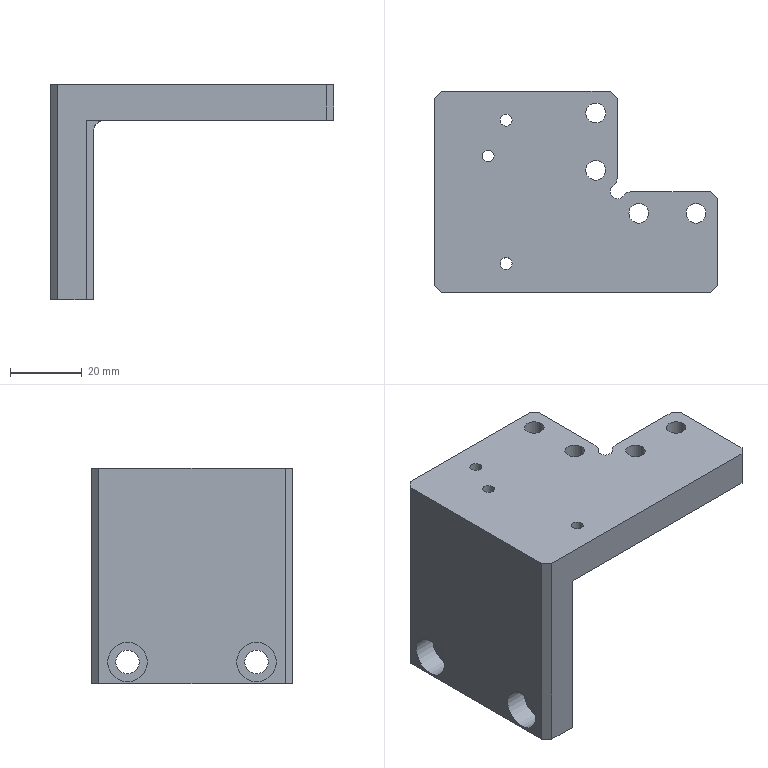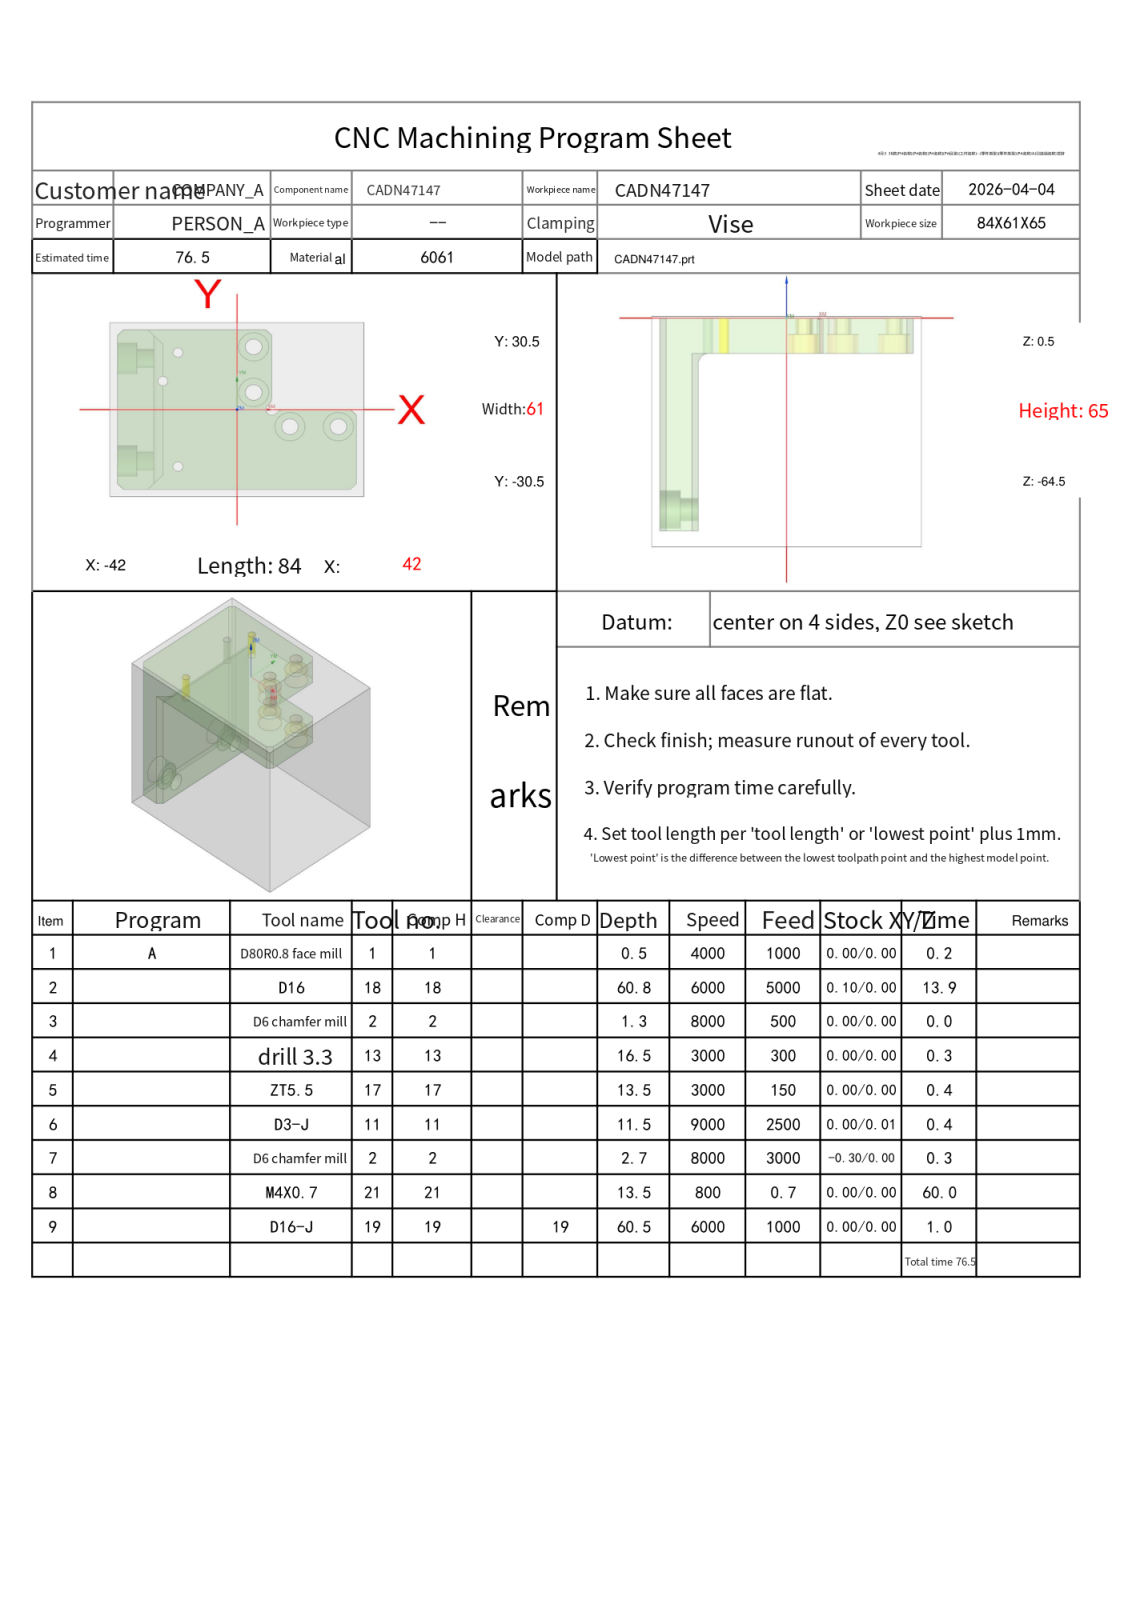NC program | NX | posted by the shop | part box 79 x 56 x 60 mm
Lines 7245 to 9053 of 9053, first 1638 of 1809 lines:
N3 T02 M06
(D6 chamfer mill  D=6. R=0. H=02 ce=0.00 di=0.00)
G00 G90 G54 X-19.5 Y-20. M03 S8000
G43 H02 Z20.
M08
G98 G81 X-19.5 Y-20. Z-.8 R1. F500.
X-24.5 Y10.
X-19.5 Y20.
X5.5 Y22.
Y6.
X17.5 Y-6.
X33.5
G80
G00 Z20.
G91 G28 Z0.0
M05
M09
G91 G28 Z0.0
M01
N4 T13 M06
(drill 3.3 D=3.3 DR_a=118 H=13)
G00 G90 G54 X-19.5 Y-20. M03 S3000
G43 H13 Z20.
M08
G98 G83 X-19.5 Y-20. Z-15.991 R1. F300. Q2.
Y20.
G80
G00 Z20.
G00 G90 X-24.5 Y10. M03 S3000
Z20.
G98 G83 X-24.5 Y10. Z-16. R1. F120. Q2.
G80
G00 Z20.
G91 G28 Z0.0
M05
M09
G91 G28 Z0.0
M01
N5 T17 M06
(ZT5.5 D=5.5 DR_a=118 H=17)
G00 G90 G54 X33.5 Y-6. M03 S3000
G43 H17 Z20.
M08
G98 G83 X33.5 Y-6. Z-13. R1. F150. Q3.
X17.5
X5.5 Y6.
Y22.
G80
G00 Z20.
G91 G28 Z0.0
M05
M09
G91 G28 Z0.0
M01
N6 T11 M06
(D3-J  D=3. R=0. H=11 ce=0.00 di=0.01)
G00 G90 G54 X13.577 Y9.224 M03 S9000
G43 H11 Z20.
M08
Z.153
G01 X13.571 Y9.223 Z.084 F2000.
X13.553 Y9.221 Z.023
X13.527 Y9.216 Z-.032
X13.491 Y9.21 Z-.081
X13.45 Y9.202 Z-.124
X13.403 Y9.191 Z-.161
X13.353 Y9.177 Z-.193
X13.3 Y9.161 Z-.22
X13.247 Y9.142 Z-.243
X13.195 Y9.119 Z-.261
X13.145 Y9.093 Z-.275
X13.099 Y9.064 Z-.285
X13.059 Y9.03 Z-.292
X13.025 Y8.993 Z-.296
X13. Y8.952 Z-.297
Y4. F2500.
G02 X11.2 Y.4 I-4.5 J0.0
G03 X11. Y0.0 I.3 J-.4
X11.5 Y-.5 I.5 J0.0
X11.9 Y-.3 I0.0 J.5
G02 X15.5 Y1.5 I3.6 J-2.7
G01 X20.452
X20.493 Y1.525 Z-.296
X20.53 Y1.559 Z-.292
X20.564 Y1.599 Z-.285
X20.593 Y1.645 Z-.275
X20.619 Y1.695 Z-.261
X20.642 Y1.747 Z-.243
X20.661 Y1.8 Z-.22
X20.677 Y1.853 Z-.193
X20.691 Y1.903 Z-.161
X20.702 Y1.95 Z-.124
X20.71 Y1.991 Z-.081
X20.716 Y2.027 Z-.032
X20.721 Y2.053 Z.023
X20.723 Y2.071 Z.084
X20.724 Y2.077 Z.153
G00 Z3.
X13.577 Y9.224
Z-.145
G01 X13.571 Y9.223 Z-.213 F2000.
X13.553 Y9.221 Z-.275
X13.527 Y9.216 Z-.33
X13.491 Y9.21 Z-.378
X13.45 Y9.202 Z-.421
X13.403 Y9.191 Z-.459
X13.353 Y9.177 Z-.49
X13.3 Y9.161 Z-.518
X13.247 Y9.142 Z-.54
X13.195 Y9.119 Z-.558
X13.145 Y9.093 Z-.572
X13.099 Y9.064 Z-.582
X13.059 Y9.03 Z-.589
X13.025 Y8.993 Z-.593
X13. Y8.952 Z-.595
Y4. F2500.
G02 X11.2 Y.4 I-4.5 J0.0
G03 X11. Y0.0 I.3 J-.4
X11.5 Y-.5 I.5 J0.0
X11.9 Y-.3 I0.0 J.5
G02 X15.5 Y1.5 I3.6 J-2.7
G01 X20.452
X20.493 Y1.525 Z-.593
X20.53 Y1.559 Z-.589
X20.564 Y1.599 Z-.582
X20.593 Y1.645 Z-.572
X20.619 Y1.695 Z-.558
X20.642 Y1.747 Z-.54
X20.661 Y1.8 Z-.518
X20.677 Y1.853 Z-.49
X20.691 Y1.903 Z-.459
X20.702 Y1.95 Z-.421
X20.71 Y1.991 Z-.378
X20.716 Y2.027 Z-.33
X20.721 Y2.053 Z-.275
X20.723 Y2.071 Z-.213
X20.724 Y2.077 Z-.145
G00 Z2.703
X13.577 Y9.224
Z-.442
G01 X13.571 Y9.223 Z-.51 F2000.
X13.553 Y9.221 Z-.572
X13.527 Y9.216 Z-.627
X13.491 Y9.21 Z-.676
X13.45 Y9.202 Z-.719
X13.403 Y9.191 Z-.756
X13.353 Y9.177 Z-.788
X13.3 Y9.161 Z-.815
X13.247 Y9.142 Z-.837
X13.195 Y9.119 Z-.855
X13.145 Y9.093 Z-.869
X13.099 Y9.064 Z-.88
X13.059 Y9.03 Z-.887
X13.025 Y8.993 Z-.891
X13. Y8.952 Z-.892
Y4. F2500.
G02 X11.2 Y.4 I-4.5 J0.0
G03 X11. Y0.0 I.3 J-.4
X11.5 Y-.5 I.5 J0.0
X11.9 Y-.3 I0.0 J.5
G02 X15.5 Y1.5 I3.6 J-2.7
G01 X20.452
X20.493 Y1.525 Z-.891
X20.53 Y1.559 Z-.887
X20.564 Y1.599 Z-.88
X20.593 Y1.645 Z-.869
X20.619 Y1.695 Z-.855
X20.642 Y1.747 Z-.837
X20.661 Y1.8 Z-.815
X20.677 Y1.853 Z-.788
X20.691 Y1.903 Z-.756
X20.702 Y1.95 Z-.719
X20.71 Y1.991 Z-.676
X20.716 Y2.027 Z-.627
X20.721 Y2.053 Z-.572
X20.723 Y2.071 Z-.51
X20.724 Y2.077 Z-.442
G00 Z2.405
X13.577 Y9.224
Z-.739
G01 X13.571 Y9.223 Z-.808 F2000.
X13.553 Y9.221 Z-.869
X13.527 Y9.216 Z-.924
X13.491 Y9.21 Z-.973
X13.45 Y9.202 Z-1.016
X13.403 Y9.191 Z-1.053
X13.353 Y9.177 Z-1.085
X13.3 Y9.161 Z-1.112
X13.247 Y9.142 Z-1.134
X13.195 Y9.119 Z-1.153
X13.145 Y9.093 Z-1.167
X13.099 Y9.064 Z-1.177
X13.059 Y9.03 Z-1.184
X13.025 Y8.993 Z-1.188
X13. Y8.952 Z-1.189
Y4. F2500.
G02 X11.2 Y.4 I-4.5 J0.0
G03 X11. Y0.0 I.3 J-.4
X11.5 Y-.5 I.5 J0.0
X11.9 Y-.3 I0.0 J.5
G02 X15.5 Y1.5 I3.6 J-2.7
G01 X20.452
X20.493 Y1.525 Z-1.188
X20.53 Y1.559 Z-1.184
X20.564 Y1.599 Z-1.177
X20.593 Y1.645 Z-1.167
X20.619 Y1.695 Z-1.153
X20.642 Y1.747 Z-1.134
X20.661 Y1.8 Z-1.112
X20.677 Y1.853 Z-1.085
X20.691 Y1.903 Z-1.053
X20.702 Y1.95 Z-1.016
X20.71 Y1.991 Z-.973
X20.716 Y2.027 Z-.924
X20.721 Y2.053 Z-.869
X20.723 Y2.071 Z-.808
X20.724 Y2.077 Z-.739
G00 Z2.108
X13.577 Y9.224
Z-1.036
G01 X13.571 Y9.223 Z-1.105 F2000.
X13.553 Y9.221 Z-1.167
X13.527 Y9.216 Z-1.222
X13.491 Y9.21 Z-1.27
X13.45 Y9.202 Z-1.313
X13.403 Y9.191 Z-1.35
X13.353 Y9.177 Z-1.382
X13.3 Y9.161 Z-1.409
X13.247 Y9.142 Z-1.432
X13.195 Y9.119 Z-1.45
X13.145 Y9.093 Z-1.464
X13.099 Y9.064 Z-1.474
X13.059 Y9.03 Z-1.481
X13.025 Y8.993 Z-1.485
X13. Y8.952 Z-1.486
Y4. F2500.
G02 X11.2 Y.4 I-4.5 J0.0
G03 X11. Y0.0 I.3 J-.4
X11.5 Y-.5 I.5 J0.0
X11.9 Y-.3 I0.0 J.5
G02 X15.5 Y1.5 I3.6 J-2.7
G01 X20.452
X20.493 Y1.525 Z-1.485
X20.53 Y1.559 Z-1.481
X20.564 Y1.599 Z-1.474
X20.593 Y1.645 Z-1.464
X20.619 Y1.695 Z-1.45
X20.642 Y1.747 Z-1.432
X20.661 Y1.8 Z-1.409
X20.677 Y1.853 Z-1.382
X20.691 Y1.903 Z-1.35
X20.702 Y1.95 Z-1.313
X20.71 Y1.991 Z-1.27
X20.716 Y2.027 Z-1.222
X20.721 Y2.053 Z-1.167
X20.723 Y2.071 Z-1.105
X20.724 Y2.077 Z-1.036
G00 Z1.811
X13.577 Y9.224
Z-1.334
G01 X13.571 Y9.223 Z-1.402 F2000.
X13.553 Y9.221 Z-1.464
X13.527 Y9.216 Z-1.519
X13.491 Y9.21 Z-1.568
X13.45 Y9.202 Z-1.61
X13.403 Y9.191 Z-1.648
X13.353 Y9.177 Z-1.68
X13.3 Y9.161 Z-1.707
X13.247 Y9.142 Z-1.729
X13.195 Y9.119 Z-1.747
X13.145 Y9.093 Z-1.761
X13.099 Y9.064 Z-1.772
X13.059 Y9.03 Z-1.779
X13.025 Y8.993 Z-1.783
X13. Y8.952 Z-1.784
Y4. F2500.
G02 X11.2 Y.4 I-4.5 J0.0
G03 X11. Y0.0 I.3 J-.4
X11.5 Y-.5 I.5 J0.0
X11.9 Y-.3 I0.0 J.5
G02 X15.5 Y1.5 I3.6 J-2.7
G01 X20.452
X20.493 Y1.525 Z-1.783
X20.53 Y1.559 Z-1.779
X20.564 Y1.599 Z-1.772
X20.593 Y1.645 Z-1.761
X20.619 Y1.695 Z-1.747
X20.642 Y1.747 Z-1.729
X20.661 Y1.8 Z-1.707
X20.677 Y1.853 Z-1.68
X20.691 Y1.903 Z-1.648
X20.702 Y1.95 Z-1.61
X20.71 Y1.991 Z-1.568
X20.716 Y2.027 Z-1.519
X20.721 Y2.053 Z-1.464
X20.723 Y2.071 Z-1.402
X20.724 Y2.077 Z-1.334
G00 Z1.514
X13.577 Y9.224
Z-1.631
G01 X13.571 Y9.223 Z-1.7 F2000.
X13.553 Y9.221 Z-1.761
X13.527 Y9.216 Z-1.816
X13.491 Y9.21 Z-1.865
X13.45 Y9.202 Z-1.908
X13.403 Y9.191 Z-1.945
X13.353 Y9.177 Z-1.977
X13.3 Y9.161 Z-2.004
X13.247 Y9.142 Z-2.026
X13.195 Y9.119 Z-2.044
X13.145 Y9.093 Z-2.058
X13.099 Y9.064 Z-2.069
X13.059 Y9.03 Z-2.076
X13.025 Y8.993 Z-2.08
X13. Y8.952 Z-2.081
Y4. F2500.
G02 X11.2 Y.4 I-4.5 J0.0
G03 X11. Y0.0 I.3 J-.4
X11.5 Y-.5 I.5 J0.0
X11.9 Y-.3 I0.0 J.5
G02 X15.5 Y1.5 I3.6 J-2.7
G01 X20.452
X20.493 Y1.525 Z-2.08
X20.53 Y1.559 Z-2.076
X20.564 Y1.599 Z-2.069
X20.593 Y1.645 Z-2.058
X20.619 Y1.695 Z-2.044
X20.642 Y1.747 Z-2.026
X20.661 Y1.8 Z-2.004
X20.677 Y1.853 Z-1.977
X20.691 Y1.903 Z-1.945
X20.702 Y1.95 Z-1.908
X20.71 Y1.991 Z-1.865
X20.716 Y2.027 Z-1.816
X20.721 Y2.053 Z-1.761
X20.723 Y2.071 Z-1.7
X20.724 Y2.077 Z-1.631
G00 Z1.216
X13.577 Y9.224
Z-1.928
G01 X13.571 Y9.223 Z-1.997 F2000.
X13.553 Y9.221 Z-2.058
X13.527 Y9.216 Z-2.113
X13.491 Y9.21 Z-2.162
X13.45 Y9.202 Z-2.205
X13.403 Y9.191 Z-2.242
X13.353 Y9.177 Z-2.274
X13.3 Y9.161 Z-2.301
X13.247 Y9.142 Z-2.324
X13.195 Y9.119 Z-2.342
X13.145 Y9.093 Z-2.356
X13.099 Y9.064 Z-2.366
X13.059 Y9.03 Z-2.373
X13.025 Y8.993 Z-2.377
X13. Y8.952 Z-2.378
Y4. F2500.
G02 X11.2 Y.4 I-4.5 J0.0
G03 X11. Y0.0 I.3 J-.4
X11.5 Y-.5 I.5 J0.0
X11.9 Y-.3 I0.0 J.5
G02 X15.5 Y1.5 I3.6 J-2.7
G01 X20.452
X20.493 Y1.525 Z-2.377
X20.53 Y1.559 Z-2.373
X20.564 Y1.599 Z-2.366
X20.593 Y1.645 Z-2.356
X20.619 Y1.695 Z-2.342
X20.642 Y1.747 Z-2.324
X20.661 Y1.8 Z-2.301
X20.677 Y1.853 Z-2.274
X20.691 Y1.903 Z-2.242
X20.702 Y1.95 Z-2.205
X20.71 Y1.991 Z-2.162
X20.716 Y2.027 Z-2.113
X20.721 Y2.053 Z-2.058
X20.723 Y2.071 Z-1.997
X20.724 Y2.077 Z-1.928
G00 Z.919
X13.577 Y9.224
Z-2.226
G01 X13.571 Y9.223 Z-2.294 F2000.
X13.553 Y9.221 Z-2.356
X13.527 Y9.216 Z-2.411
X13.491 Y9.21 Z-2.459
X13.45 Y9.202 Z-2.502
X13.403 Y9.191 Z-2.54
X13.353 Y9.177 Z-2.572
X13.3 Y9.161 Z-2.599
X13.247 Y9.142 Z-2.621
X13.195 Y9.119 Z-2.639
X13.145 Y9.093 Z-2.653
X13.099 Y9.064 Z-2.663
X13.059 Y9.03 Z-2.67
X13.025 Y8.993 Z-2.674
X13. Y8.952 Z-2.676
Y4. F2500.
G02 X11.2 Y.4 I-4.5 J0.0
G03 X11. Y0.0 I.3 J-.4
X11.5 Y-.5 I.5 J0.0
X11.9 Y-.3 I0.0 J.5
G02 X15.5 Y1.5 I3.6 J-2.7
G01 X20.452
X20.493 Y1.525 Z-2.674
X20.53 Y1.559 Z-2.67
X20.564 Y1.599 Z-2.663
X20.593 Y1.645 Z-2.653
X20.619 Y1.695 Z-2.639
X20.642 Y1.747 Z-2.621
X20.661 Y1.8 Z-2.599
X20.677 Y1.853 Z-2.572
X20.691 Y1.903 Z-2.54
X20.702 Y1.95 Z-2.502
X20.71 Y1.991 Z-2.459
X20.716 Y2.027 Z-2.411
X20.721 Y2.053 Z-2.356
X20.723 Y2.071 Z-2.294
X20.724 Y2.077 Z-2.226
G00 Z.622
X13.577 Y9.224
Z-2.523
G01 X13.571 Y9.223 Z-2.591 F2000.
X13.553 Y9.221 Z-2.653
X13.527 Y9.216 Z-2.708
X13.491 Y9.21 Z-2.757
X13.45 Y9.202 Z-2.8
X13.403 Y9.191 Z-2.837
X13.353 Y9.177 Z-2.869
X13.3 Y9.161 Z-2.896
X13.247 Y9.142 Z-2.918
X13.195 Y9.119 Z-2.936
X13.145 Y9.093 Z-2.95
X13.099 Y9.064 Z-2.961
X13.059 Y9.03 Z-2.968
X13.025 Y8.993 Z-2.972
X13. Y8.952 Z-2.973
Y4. F2500.
G02 X11.2 Y.4 I-4.5 J0.0
G03 X11. Y0.0 I.3 J-.4
X11.5 Y-.5 I.5 J0.0
X11.9 Y-.3 I0.0 J.5
G02 X15.5 Y1.5 I3.6 J-2.7
G01 X20.452
X20.493 Y1.525 Z-2.972
X20.53 Y1.559 Z-2.968
X20.564 Y1.599 Z-2.961
X20.593 Y1.645 Z-2.95
X20.619 Y1.695 Z-2.936
X20.642 Y1.747 Z-2.918
X20.661 Y1.8 Z-2.896
X20.677 Y1.853 Z-2.869
X20.691 Y1.903 Z-2.837
X20.702 Y1.95 Z-2.8
X20.71 Y1.991 Z-2.757
X20.716 Y2.027 Z-2.708
X20.721 Y2.053 Z-2.653
X20.723 Y2.071 Z-2.591
X20.724 Y2.077 Z-2.523
G00 Z.324
X13.577 Y9.224
Z-2.82
G01 X13.571 Y9.223 Z-2.889 F2000.
X13.553 Y9.221 Z-2.95
X13.527 Y9.216 Z-3.005
X13.491 Y9.21 Z-3.054
X13.45 Y9.202 Z-3.097
X13.403 Y9.191 Z-3.134
X13.353 Y9.177 Z-3.166
X13.3 Y9.161 Z-3.193
X13.247 Y9.142 Z-3.216
X13.195 Y9.119 Z-3.234
X13.145 Y9.093 Z-3.248
X13.099 Y9.064 Z-3.258
X13.059 Y9.03 Z-3.265
X13.025 Y8.993 Z-3.269
X13. Y8.952 Z-3.27
Y4. F2500.
G02 X11.2 Y.4 I-4.5 J0.0
G03 X11. Y0.0 I.3 J-.4
X11.5 Y-.5 I.5 J0.0
X11.9 Y-.3 I0.0 J.5
G02 X15.5 Y1.5 I3.6 J-2.7
G01 X20.452
X20.493 Y1.525 Z-3.269
X20.53 Y1.559 Z-3.265
X20.564 Y1.599 Z-3.258
X20.593 Y1.645 Z-3.248
X20.619 Y1.695 Z-3.234
X20.642 Y1.747 Z-3.216
X20.661 Y1.8 Z-3.193
X20.677 Y1.853 Z-3.166
X20.691 Y1.903 Z-3.134
X20.702 Y1.95 Z-3.097
X20.71 Y1.991 Z-3.054
X20.716 Y2.027 Z-3.005
X20.721 Y2.053 Z-2.95
X20.723 Y2.071 Z-2.889
X20.724 Y2.077 Z-2.82
G00 Z.027
X13.577 Y9.224
Z-3.118
G01 X13.571 Y9.223 Z-3.186 F2000.
X13.553 Y9.221 Z-3.248
X13.527 Y9.216 Z-3.303
X13.491 Y9.21 Z-3.351
X13.45 Y9.202 Z-3.394
X13.403 Y9.191 Z-3.431
X13.353 Y9.177 Z-3.463
X13.3 Y9.161 Z-3.49
X13.247 Y9.142 Z-3.513
X13.195 Y9.119 Z-3.531
X13.145 Y9.093 Z-3.545
X13.099 Y9.064 Z-3.555
X13.059 Y9.03 Z-3.562
X13.025 Y8.993 Z-3.566
X13. Y8.952 Z-3.568
Y4. F2500.
G02 X11.2 Y.4 I-4.5 J0.0
G03 X11. Y0.0 I.3 J-.4
X11.5 Y-.5 I.5 J0.0
X11.9 Y-.3 I0.0 J.5
G02 X15.5 Y1.5 I3.6 J-2.7
G01 X20.452
X20.493 Y1.525 Z-3.566
X20.53 Y1.559 Z-3.562
X20.564 Y1.599 Z-3.555
X20.593 Y1.645 Z-3.545
X20.619 Y1.695 Z-3.531
X20.642 Y1.747 Z-3.513
X20.661 Y1.8 Z-3.49
X20.677 Y1.853 Z-3.463
X20.691 Y1.903 Z-3.431
X20.702 Y1.95 Z-3.394
X20.71 Y1.991 Z-3.351
X20.716 Y2.027 Z-3.303
X20.721 Y2.053 Z-3.248
X20.723 Y2.071 Z-3.186
X20.724 Y2.077 Z-3.118
G00 Z-.27
X13.577 Y9.224
Z-3.415
G01 X13.571 Y9.223 Z-3.483 F2000.
X13.553 Y9.221 Z-3.545
X13.527 Y9.216 Z-3.6
X13.491 Y9.21 Z-3.649
X13.45 Y9.202 Z-3.692
X13.403 Y9.191 Z-3.729
X13.353 Y9.177 Z-3.761
X13.3 Y9.161 Z-3.788
X13.247 Y9.142 Z-3.81
X13.195 Y9.119 Z-3.828
X13.145 Y9.093 Z-3.842
X13.099 Y9.064 Z-3.853
X13.059 Y9.03 Z-3.86
X13.025 Y8.993 Z-3.864
X13. Y8.952 Z-3.865
Y4. F2500.
G02 X11.2 Y.4 I-4.5 J0.0
G03 X11. Y0.0 I.3 J-.4
X11.5 Y-.5 I.5 J0.0
X11.9 Y-.3 I0.0 J.5
G02 X15.5 Y1.5 I3.6 J-2.7
G01 X20.452
X20.493 Y1.525 Z-3.864
X20.53 Y1.559 Z-3.86
X20.564 Y1.599 Z-3.853
X20.593 Y1.645 Z-3.842
X20.619 Y1.695 Z-3.828
X20.642 Y1.747 Z-3.81
X20.661 Y1.8 Z-3.788
X20.677 Y1.853 Z-3.761
X20.691 Y1.903 Z-3.729
X20.702 Y1.95 Z-3.692
X20.71 Y1.991 Z-3.649
X20.716 Y2.027 Z-3.6
X20.721 Y2.053 Z-3.545
X20.723 Y2.071 Z-3.483
X20.724 Y2.077 Z-3.415
G00 Z-.568
X13.577 Y9.224
Z-3.712
G01 X13.571 Y9.223 Z-3.781 F2000.
X13.553 Y9.221 Z-3.842
X13.527 Y9.216 Z-3.897
X13.491 Y9.21 Z-3.946
X13.45 Y9.202 Z-3.989
X13.403 Y9.191 Z-4.026
X13.353 Y9.177 Z-4.058
X13.3 Y9.161 Z-4.085
X13.247 Y9.142 Z-4.107
X13.195 Y9.119 Z-4.125
X13.145 Y9.093 Z-4.14
X13.099 Y9.064 Z-4.15
X13.059 Y9.03 Z-4.157
X13.025 Y8.993 Z-4.161
X13. Y8.952 Z-4.162
Y4. F2500.
G02 X11.2 Y.4 I-4.5 J0.0
G03 X11. Y0.0 I.3 J-.4
X11.5 Y-.5 I.5 J0.0
X11.9 Y-.3 I0.0 J.5
G02 X15.5 Y1.5 I3.6 J-2.7
G01 X20.452
X20.493 Y1.525 Z-4.161
X20.53 Y1.559 Z-4.157
X20.564 Y1.599 Z-4.15
X20.593 Y1.645 Z-4.14
X20.619 Y1.695 Z-4.125
X20.642 Y1.747 Z-4.107
X20.661 Y1.8 Z-4.085
X20.677 Y1.853 Z-4.058
X20.691 Y1.903 Z-4.026
X20.702 Y1.95 Z-3.989
X20.71 Y1.991 Z-3.946
X20.716 Y2.027 Z-3.897
X20.721 Y2.053 Z-3.842
X20.723 Y2.071 Z-3.781
X20.724 Y2.077 Z-3.712
G00 Z-.865
X13.577 Y9.224
Z-4.009
G01 X13.571 Y9.223 Z-4.078 F2000.
X13.553 Y9.221 Z-4.139
X13.527 Y9.216 Z-4.195
X13.491 Y9.21 Z-4.243
X13.45 Y9.202 Z-4.286
X13.403 Y9.191 Z-4.323
X13.353 Y9.177 Z-4.355
X13.3 Y9.161 Z-4.382
X13.247 Y9.142 Z-4.405
X13.195 Y9.119 Z-4.423
X13.145 Y9.093 Z-4.437
X13.099 Y9.064 Z-4.447
X13.059 Y9.03 Z-4.454
X13.025 Y8.993 Z-4.458
X13. Y8.952 Z-4.459
Y4. F2500.
G02 X11.2 Y.4 I-4.5 J0.0
G03 X11. Y0.0 I.3 J-.4
X11.5 Y-.5 I.5 J0.0
X11.9 Y-.3 I0.0 J.5
G02 X15.5 Y1.5 I3.6 J-2.7
G01 X20.452
X20.493 Y1.525 Z-4.458
X20.53 Y1.559 Z-4.454
X20.564 Y1.599 Z-4.447
X20.593 Y1.645 Z-4.437
X20.619 Y1.695 Z-4.423
X20.642 Y1.747 Z-4.405
X20.661 Y1.8 Z-4.382
X20.677 Y1.853 Z-4.355
X20.691 Y1.903 Z-4.323
X20.702 Y1.95 Z-4.286
X20.71 Y1.991 Z-4.243
X20.716 Y2.027 Z-4.195
X20.721 Y2.053 Z-4.139
X20.723 Y2.071 Z-4.078
X20.724 Y2.077 Z-4.009
G00 Z-1.162
X13.577 Y9.224
Z-4.307
G01 X13.571 Y9.223 Z-4.375 F2000.
X13.553 Y9.221 Z-4.437
X13.527 Y9.216 Z-4.492
X13.491 Y9.21 Z-4.541
X13.45 Y9.202 Z-4.583
X13.403 Y9.191 Z-4.621
X13.353 Y9.177 Z-4.653
X13.3 Y9.161 Z-4.68
X13.247 Y9.142 Z-4.702
X13.195 Y9.119 Z-4.72
X13.145 Y9.093 Z-4.734
X13.099 Y9.064 Z-4.745
X13.059 Y9.03 Z-4.752
X13.025 Y8.993 Z-4.756
X13. Y8.952 Z-4.757
Y4. F2500.
G02 X11.2 Y.4 I-4.5 J0.0
G03 X11. Y0.0 I.3 J-.4
X11.5 Y-.5 I.5 J0.0
X11.9 Y-.3 I0.0 J.5
G02 X15.5 Y1.5 I3.6 J-2.7
G01 X20.452
X20.493 Y1.525 Z-4.756
X20.53 Y1.559 Z-4.752
X20.564 Y1.599 Z-4.745
X20.593 Y1.645 Z-4.734
X20.619 Y1.695 Z-4.72
X20.642 Y1.747 Z-4.702
X20.661 Y1.8 Z-4.68
X20.677 Y1.853 Z-4.653
X20.691 Y1.903 Z-4.621
X20.702 Y1.95 Z-4.583
X20.71 Y1.991 Z-4.541
X20.716 Y2.027 Z-4.492
X20.721 Y2.053 Z-4.437
X20.723 Y2.071 Z-4.375
X20.724 Y2.077 Z-4.307
G00 Z-1.459
X13.577 Y9.224
Z-4.604
G01 X13.571 Y9.223 Z-4.673 F2000.
X13.553 Y9.221 Z-4.734
X13.527 Y9.216 Z-4.789
X13.491 Y9.21 Z-4.838
X13.45 Y9.202 Z-4.881
X13.403 Y9.191 Z-4.918
X13.353 Y9.177 Z-4.95
X13.3 Y9.161 Z-4.977
X13.247 Y9.142 Z-4.999
X13.195 Y9.119 Z-5.017
X13.145 Y9.093 Z-5.031
X13.099 Y9.064 Z-5.042
X13.059 Y9.03 Z-5.049
X13.025 Y8.993 Z-5.053
X13. Y8.952 Z-5.054
Y4. F2500.
G02 X11.2 Y.4 I-4.5 J0.0
G03 X11. Y0.0 I.3 J-.4
X11.5 Y-.5 I.5 J0.0
X11.9 Y-.3 I0.0 J.5
G02 X15.5 Y1.5 I3.6 J-2.7
G01 X20.452
X20.493 Y1.525 Z-5.053
X20.53 Y1.559 Z-5.049
X20.564 Y1.599 Z-5.042
X20.593 Y1.645 Z-5.031
X20.619 Y1.695 Z-5.017
X20.642 Y1.747 Z-4.999
X20.661 Y1.8 Z-4.977
X20.677 Y1.853 Z-4.95
X20.691 Y1.903 Z-4.918
X20.702 Y1.95 Z-4.881
X20.71 Y1.991 Z-4.838
X20.716 Y2.027 Z-4.789
X20.721 Y2.053 Z-4.734
X20.723 Y2.071 Z-4.673
X20.724 Y2.077 Z-4.604
G00 Z-1.757
X13.577 Y9.224
Z-4.901
G01 X13.571 Y9.223 Z-4.97 F2000.
X13.553 Y9.221 Z-5.031
X13.527 Y9.216 Z-5.086
X13.491 Y9.21 Z-5.135
X13.45 Y9.202 Z-5.178
X13.403 Y9.191 Z-5.215
X13.353 Y9.177 Z-5.247
X13.3 Y9.161 Z-5.274
X13.247 Y9.142 Z-5.297
X13.195 Y9.119 Z-5.315
X13.145 Y9.093 Z-5.329
X13.099 Y9.064 Z-5.339
X13.059 Y9.03 Z-5.346
X13.025 Y8.993 Z-5.35
X13. Y8.952 Z-5.351
Y4. F2500.
G02 X11.2 Y.4 I-4.5 J0.0
G03 X11. Y0.0 I.3 J-.4
X11.5 Y-.5 I.5 J0.0
X11.9 Y-.3 I0.0 J.5
G02 X15.5 Y1.5 I3.6 J-2.7
G01 X20.452
X20.493 Y1.525 Z-5.35
X20.53 Y1.559 Z-5.346
X20.564 Y1.599 Z-5.339
X20.593 Y1.645 Z-5.329
X20.619 Y1.695 Z-5.315
X20.642 Y1.747 Z-5.297
X20.661 Y1.8 Z-5.274
X20.677 Y1.853 Z-5.247
X20.691 Y1.903 Z-5.215
X20.702 Y1.95 Z-5.178
X20.71 Y1.991 Z-5.135
X20.716 Y2.027 Z-5.086
X20.721 Y2.053 Z-5.031
X20.723 Y2.071 Z-4.97
X20.724 Y2.077 Z-4.901
G00 Z-2.054
X13.577 Y9.224
Z-5.199
G01 X13.571 Y9.223 Z-5.267 F2000.
X13.553 Y9.221 Z-5.329
X13.527 Y9.216 Z-5.384
X13.491 Y9.21 Z-5.432
X13.45 Y9.202 Z-5.475
X13.403 Y9.191 Z-5.513
X13.353 Y9.177 Z-5.545
X13.3 Y9.161 Z-5.572
X13.247 Y9.142 Z-5.594
X13.195 Y9.119 Z-5.612
X13.145 Y9.093 Z-5.626
X13.099 Y9.064 Z-5.636
X13.059 Y9.03 Z-5.643
X13.025 Y8.993 Z-5.647
X13. Y8.952 Z-5.649
Y4. F2500.
G02 X11.2 Y.4 I-4.5 J0.0
G03 X11. Y0.0 I.3 J-.4
X11.5 Y-.5 I.5 J0.0
X11.9 Y-.3 I0.0 J.5
G02 X15.5 Y1.5 I3.6 J-2.7
G01 X20.452
X20.493 Y1.525 Z-5.647
X20.53 Y1.559 Z-5.643
X20.564 Y1.599 Z-5.636
X20.593 Y1.645 Z-5.626
X20.619 Y1.695 Z-5.612
X20.642 Y1.747 Z-5.594
X20.661 Y1.8 Z-5.572
X20.677 Y1.853 Z-5.545
X20.691 Y1.903 Z-5.513
X20.702 Y1.95 Z-5.475
X20.71 Y1.991 Z-5.432
X20.716 Y2.027 Z-5.384
X20.721 Y2.053 Z-5.329
X20.723 Y2.071 Z-5.267
X20.724 Y2.077 Z-5.199
G00 Z-2.351
X13.577 Y9.224
Z-5.496
G01 X13.571 Y9.223 Z-5.564 F2000.
X13.553 Y9.221 Z-5.626
X13.527 Y9.216 Z-5.681
X13.491 Y9.21 Z-5.73
X13.45 Y9.202 Z-5.773
X13.403 Y9.191 Z-5.81
X13.353 Y9.177 Z-5.842
X13.3 Y9.161 Z-5.869
X13.247 Y9.142 Z-5.891
X13.195 Y9.119 Z-5.909
X13.145 Y9.093 Z-5.923
X13.099 Y9.064 Z-5.934
X13.059 Y9.03 Z-5.941
X13.025 Y8.993 Z-5.945
X13. Y8.952 Z-5.946
Y4. F2500.
G02 X11.2 Y.4 I-4.5 J0.0
G03 X11. Y0.0 I.3 J-.4
X11.5 Y-.5 I.5 J0.0
X11.9 Y-.3 I0.0 J.5
G02 X15.5 Y1.5 I3.6 J-2.7
G01 X20.452
X20.493 Y1.525 Z-5.945
X20.53 Y1.559 Z-5.941
X20.564 Y1.599 Z-5.934
X20.593 Y1.645 Z-5.923
X20.619 Y1.695 Z-5.909
X20.642 Y1.747 Z-5.891
X20.661 Y1.8 Z-5.869
X20.677 Y1.853 Z-5.842
X20.691 Y1.903 Z-5.81
X20.702 Y1.95 Z-5.773
X20.71 Y1.991 Z-5.73
X20.716 Y2.027 Z-5.681
X20.721 Y2.053 Z-5.626
X20.723 Y2.071 Z-5.564
X20.724 Y2.077 Z-5.496
G00 Z-2.649
X13.577 Y9.224
Z-5.793
G01 X13.571 Y9.223 Z-5.862 F2000.
X13.553 Y9.221 Z-5.923
X13.527 Y9.216 Z-5.978
X13.491 Y9.21 Z-6.027
X13.45 Y9.202 Z-6.07
X13.403 Y9.191 Z-6.107
X13.353 Y9.177 Z-6.139
X13.3 Y9.161 Z-6.166
X13.247 Y9.142 Z-6.189
X13.195 Y9.119 Z-6.207
X13.145 Y9.093 Z-6.221
X13.099 Y9.064 Z-6.231
X13.059 Y9.03 Z-6.238
X13.025 Y8.993 Z-6.242
X13. Y8.952 Z-6.243
Y4. F2500.
G02 X11.2 Y.4 I-4.5 J0.0
G03 X11. Y0.0 I.3 J-.4
X11.5 Y-.5 I.5 J0.0
X11.9 Y-.3 I0.0 J.5
G02 X15.5 Y1.5 I3.6 J-2.7
G01 X20.452
X20.493 Y1.525 Z-6.242
X20.53 Y1.559 Z-6.238
X20.564 Y1.599 Z-6.231
X20.593 Y1.645 Z-6.221
X20.619 Y1.695 Z-6.207
X20.642 Y1.747 Z-6.189
X20.661 Y1.8 Z-6.166
X20.677 Y1.853 Z-6.139
X20.691 Y1.903 Z-6.107
X20.702 Y1.95 Z-6.07
X20.71 Y1.991 Z-6.027
X20.716 Y2.027 Z-5.978
X20.721 Y2.053 Z-5.923
X20.723 Y2.071 Z-5.862
X20.724 Y2.077 Z-5.793
G00 Z-2.946
X13.577 Y9.224
Z-6.091
G01 X13.571 Y9.223 Z-6.159 F2000.
X13.553 Y9.221 Z-6.221
X13.527 Y9.216 Z-6.276
X13.491 Y9.21 Z-6.324
X13.45 Y9.202 Z-6.367
X13.403 Y9.191 Z-6.404
X13.353 Y9.177 Z-6.436
X13.3 Y9.161 Z-6.463
X13.247 Y9.142 Z-6.486
X13.195 Y9.119 Z-6.504
X13.145 Y9.093 Z-6.518
X13.099 Y9.064 Z-6.528
X13.059 Y9.03 Z-6.535
X13.025 Y8.993 Z-6.539
X13. Y8.952 Z-6.541
Y4. F2500.
G02 X11.2 Y.4 I-4.5 J0.0
G03 X11. Y0.0 I.3 J-.4
X11.5 Y-.5 I.5 J0.0
X11.9 Y-.3 I0.0 J.5
G02 X15.5 Y1.5 I3.6 J-2.7
G01 X20.452
X20.493 Y1.525 Z-6.539
X20.53 Y1.559 Z-6.535
X20.564 Y1.599 Z-6.528
X20.593 Y1.645 Z-6.518
X20.619 Y1.695 Z-6.504
X20.642 Y1.747 Z-6.486
X20.661 Y1.8 Z-6.463
X20.677 Y1.853 Z-6.436
X20.691 Y1.903 Z-6.404
X20.702 Y1.95 Z-6.367
X20.71 Y1.991 Z-6.324
X20.716 Y2.027 Z-6.276
X20.721 Y2.053 Z-6.221
X20.723 Y2.071 Z-6.159
X20.724 Y2.077 Z-6.091
G00 Z-3.243
X13.577 Y9.224
Z-6.388
G01 X13.571 Y9.223 Z-6.456 F2000.
X13.553 Y9.221 Z-6.518
X13.527 Y9.216 Z-6.573
X13.491 Y9.21 Z-6.622
X13.45 Y9.202 Z-6.665
X13.403 Y9.191 Z-6.702
X13.353 Y9.177 Z-6.734
X13.3 Y9.161 Z-6.761
X13.247 Y9.142 Z-6.783
X13.195 Y9.119 Z-6.801
X13.145 Y9.093 Z-6.815
X13.099 Y9.064 Z-6.826
X13.059 Y9.03 Z-6.833
X13.025 Y8.993 Z-6.837
X13. Y8.952 Z-6.838
Y4. F2500.
G02 X11.2 Y.4 I-4.5 J0.0
G03 X11. Y0.0 I.3 J-.4
X11.5 Y-.5 I.5 J0.0
X11.9 Y-.3 I0.0 J.5
G02 X15.5 Y1.5 I3.6 J-2.7
G01 X20.452
X20.493 Y1.525 Z-6.837
X20.53 Y1.559 Z-6.833
X20.564 Y1.599 Z-6.826
X20.593 Y1.645 Z-6.815
X20.619 Y1.695 Z-6.801
X20.642 Y1.747 Z-6.783
X20.661 Y1.8 Z-6.761
X20.677 Y1.853 Z-6.734
X20.691 Y1.903 Z-6.702
X20.702 Y1.95 Z-6.665
X20.71 Y1.991 Z-6.622
X20.716 Y2.027 Z-6.573
X20.721 Y2.053 Z-6.518
X20.723 Y2.071 Z-6.456
X20.724 Y2.077 Z-6.388
G00 Z-3.541
X13.577 Y9.224
Z-6.685
G01 X13.571 Y9.223 Z-6.754 F2000.
X13.553 Y9.221 Z-6.815
X13.527 Y9.216 Z-6.87
X13.491 Y9.21 Z-6.919
X13.45 Y9.202 Z-6.962
X13.403 Y9.191 Z-6.999
X13.353 Y9.177 Z-7.031
X13.3 Y9.161 Z-7.058
X13.247 Y9.142 Z-7.08
X13.195 Y9.119 Z-7.098
X13.145 Y9.093 Z-7.113
X13.099 Y9.064 Z-7.123
X13.059 Y9.03 Z-7.13
X13.025 Y8.993 Z-7.134
X13. Y8.952 Z-7.135
Y4. F2500.
G02 X11.2 Y.4 I-4.5 J0.0
G03 X11. Y0.0 I.3 J-.4
X11.5 Y-.5 I.5 J0.0
X11.9 Y-.3 I0.0 J.5
G02 X15.5 Y1.5 I3.6 J-2.7
G01 X20.452
X20.493 Y1.525 Z-7.134
X20.53 Y1.559 Z-7.13
X20.564 Y1.599 Z-7.123
X20.593 Y1.645 Z-7.113
X20.619 Y1.695 Z-7.098
X20.642 Y1.747 Z-7.08
X20.661 Y1.8 Z-7.058
X20.677 Y1.853 Z-7.031
X20.691 Y1.903 Z-6.999
X20.702 Y1.95 Z-6.962
X20.71 Y1.991 Z-6.919
X20.716 Y2.027 Z-6.87
X20.721 Y2.053 Z-6.815
X20.723 Y2.071 Z-6.754
X20.724 Y2.077 Z-6.685
G00 Z-3.838
X13.577 Y9.224
Z-6.982
G01 X13.571 Y9.223 Z-7.051 F2000.
X13.553 Y9.221 Z-7.112
X13.527 Y9.216 Z-7.167
X13.491 Y9.21 Z-7.216
X13.45 Y9.202 Z-7.259
X13.403 Y9.191 Z-7.296
X13.353 Y9.177 Z-7.328
X13.3 Y9.161 Z-7.355
X13.247 Y9.142 Z-7.378
X13.195 Y9.119 Z-7.396
X13.145 Y9.093 Z-7.41
X13.099 Y9.064 Z-7.42
X13.059 Y9.03 Z-7.427
X13.025 Y8.993 Z-7.431
X13. Y8.952 Z-7.432
Y4. F2500.
G02 X11.2 Y.4 I-4.5 J0.0
G03 X11. Y0.0 I.3 J-.4
X11.5 Y-.5 I.5 J0.0
X11.9 Y-.3 I0.0 J.5
G02 X15.5 Y1.5 I3.6 J-2.7
G01 X20.452
X20.493 Y1.525 Z-7.431
X20.53 Y1.559 Z-7.427
X20.564 Y1.599 Z-7.42
X20.593 Y1.645 Z-7.41
X20.619 Y1.695 Z-7.396
X20.642 Y1.747 Z-7.378
X20.661 Y1.8 Z-7.355
X20.677 Y1.853 Z-7.328
X20.691 Y1.903 Z-7.296
X20.702 Y1.95 Z-7.259
X20.71 Y1.991 Z-7.216
X20.716 Y2.027 Z-7.167
X20.721 Y2.053 Z-7.112
X20.723 Y2.071 Z-7.051
X20.724 Y2.077 Z-6.982
G00 Z-4.135
X13.577 Y9.224
Z-7.28
G01 X13.571 Y9.223 Z-7.348 F2000.
X13.553 Y9.221 Z-7.41
X13.527 Y9.216 Z-7.465
X13.491 Y9.21 Z-7.514
X13.45 Y9.202 Z-7.556
X13.403 Y9.191 Z-7.594
X13.353 Y9.177 Z-7.626
X13.3 Y9.161 Z-7.653
X13.247 Y9.142 Z-7.675
X13.195 Y9.119 Z-7.693
X13.145 Y9.093 Z-7.707
X13.099 Y9.064 Z-7.717
X13.059 Y9.03 Z-7.725
X13.025 Y8.993 Z-7.728
X13. Y8.952 Z-7.73
Y4. F2500.
G02 X11.2 Y.4 I-4.5 J0.0
G03 X11. Y0.0 I.3 J-.4
X11.5 Y-.5 I.5 J0.0
X11.9 Y-.3 I0.0 J.5
G02 X15.5 Y1.5 I3.6 J-2.7
G01 X20.452
X20.493 Y1.525 Z-7.728
X20.53 Y1.559 Z-7.725
X20.564 Y1.599 Z-7.717
X20.593 Y1.645 Z-7.707
X20.619 Y1.695 Z-7.693
X20.642 Y1.747 Z-7.675
X20.661 Y1.8 Z-7.653
X20.677 Y1.853 Z-7.626
X20.691 Y1.903 Z-7.594
X20.702 Y1.95 Z-7.556
X20.71 Y1.991 Z-7.514
X20.716 Y2.027 Z-7.465
X20.721 Y2.053 Z-7.41
X20.723 Y2.071 Z-7.348
X20.724 Y2.077 Z-7.28
G00 Z-4.432
X13.577 Y9.224
Z-7.577
G01 X13.571 Y9.223 Z-7.645 F2000.
X13.553 Y9.221 Z-7.707
X13.527 Y9.216 Z-7.762
X13.491 Y9.21 Z-7.811
X13.45 Y9.202 Z-7.854
X13.403 Y9.191 Z-7.891
X13.353 Y9.177 Z-7.923
X13.3 Y9.161 Z-7.95
X13.247 Y9.142 Z-7.972
X13.195 Y9.119 Z-7.99
X13.145 Y9.093 Z-8.004
X13.099 Y9.064 Z-8.015
X13.059 Y9.03 Z-8.022
X13.025 Y8.993 Z-8.026
X13. Y8.952 Z-8.027
Y4. F2500.
G02 X11.2 Y.4 I-4.5 J0.0
G03 X11. Y0.0 I.3 J-.4
X11.5 Y-.5 I.5 J0.0
X11.9 Y-.3 I0.0 J.5
G02 X15.5 Y1.5 I3.6 J-2.7
G01 X20.452
X20.493 Y1.525 Z-8.026
X20.53 Y1.559 Z-8.022
X20.564 Y1.599 Z-8.015
X20.593 Y1.645 Z-8.004
X20.619 Y1.695 Z-7.99
X20.642 Y1.747 Z-7.972
X20.661 Y1.8 Z-7.95
X20.677 Y1.853 Z-7.923
X20.691 Y1.903 Z-7.891
X20.702 Y1.95 Z-7.854
X20.71 Y1.991 Z-7.811
X20.716 Y2.027 Z-7.762
X20.721 Y2.053 Z-7.707
X20.723 Y2.071 Z-7.645
X20.724 Y2.077 Z-7.577
G00 Z-4.73
X13.577 Y9.224
Z-7.874
G01 X13.571 Y9.223 Z-7.943 F2000.
X13.553 Y9.221 Z-8.004
X13.527 Y9.216 Z-8.059
X13.491 Y9.21 Z-8.108
X13.45 Y9.202 Z-8.151
X13.403 Y9.191 Z-8.188
X13.353 Y9.177 Z-8.22
X13.3 Y9.161 Z-8.247
X13.247 Y9.142 Z-8.27
X13.195 Y9.119 Z-8.288
X13.145 Y9.093 Z-8.302
X13.099 Y9.064 Z-8.312
X13.059 Y9.03 Z-8.319
X13.025 Y8.993 Z-8.323
X13. Y8.952 Z-8.324
Y4. F2500.
G02 X11.2 Y.4 I-4.5 J0.0
G03 X11. Y0.0 I.3 J-.4
X11.5 Y-.5 I.5 J0.0
X11.9 Y-.3 I0.0 J.5
G02 X15.5 Y1.5 I3.6 J-2.7
G01 X20.452
X20.493 Y1.525 Z-8.323
X20.53 Y1.559 Z-8.319
X20.564 Y1.599 Z-8.312
X20.593 Y1.645 Z-8.302
X20.619 Y1.695 Z-8.288
X20.642 Y1.747 Z-8.27
X20.661 Y1.8 Z-8.247
X20.677 Y1.853 Z-8.22
X20.691 Y1.903 Z-8.188
X20.702 Y1.95 Z-8.151
X20.71 Y1.991 Z-8.108
X20.716 Y2.027 Z-8.059
X20.721 Y2.053 Z-8.004
X20.723 Y2.071 Z-7.943
X20.724 Y2.077 Z-7.874
G00 Z-5.027
X13.577 Y9.224
Z-8.172
G01 X13.571 Y9.223 Z-8.24 F2000.
X13.553 Y9.221 Z-8.302
X13.527 Y9.216 Z-8.357
X13.491 Y9.21 Z-8.405
X13.45 Y9.202 Z-8.448
X13.403 Y9.191 Z-8.486
X13.353 Y9.177 Z-8.518
X13.3 Y9.161 Z-8.545
X13.247 Y9.142 Z-8.567
X13.195 Y9.119 Z-8.585
X13.145 Y9.093 Z-8.599
X13.099 Y9.064 Z-8.609
X13.059 Y9.03 Z-8.616
X13.025 Y8.993 Z-8.62
X13. Y8.952 Z-8.622
Y4. F2500.
G02 X11.2 Y.4 I-4.5 J0.0
G03 X11. Y0.0 I.3 J-.4
X11.5 Y-.5 I.5 J0.0
X11.9 Y-.3 I0.0 J.5
G02 X15.5 Y1.5 I3.6 J-2.7
G01 X20.452
X20.493 Y1.525 Z-8.62
X20.53 Y1.559 Z-8.616
X20.564 Y1.599 Z-8.609
X20.593 Y1.645 Z-8.599
X20.619 Y1.695 Z-8.585
X20.642 Y1.747 Z-8.567
X20.661 Y1.8 Z-8.545
X20.677 Y1.853 Z-8.518
X20.691 Y1.903 Z-8.486
X20.702 Y1.95 Z-8.448
X20.71 Y1.991 Z-8.405
X20.716 Y2.027 Z-8.357
X20.721 Y2.053 Z-8.302
X20.723 Y2.071 Z-8.24
X20.724 Y2.077 Z-8.172
G00 Z-5.324
X13.577 Y9.224
Z-8.469
G01 X13.571 Y9.223 Z-8.537 F2000.
X13.553 Y9.221 Z-8.599
X13.527 Y9.216 Z-8.654
X13.491 Y9.21 Z-8.703
X13.45 Y9.202 Z-8.746
X13.403 Y9.191 Z-8.783
X13.353 Y9.177 Z-8.815
X13.3 Y9.161 Z-8.842
X13.247 Y9.142 Z-8.864
X13.195 Y9.119 Z-8.882
X13.145 Y9.093 Z-8.896
X13.099 Y9.064 Z-8.907
X13.059 Y9.03 Z-8.914
X13.025 Y8.993 Z-8.918
X13. Y8.952 Z-8.919
Y4. F2500.
G02 X11.2 Y.4 I-4.5 J0.0
G03 X11. Y0.0 I.3 J-.4
X11.5 Y-.5 I.5 J0.0
X11.9 Y-.3 I0.0 J.5
G02 X15.5 Y1.5 I3.6 J-2.7
G01 X20.452
X20.493 Y1.525 Z-8.918
X20.53 Y1.559 Z-8.914
X20.564 Y1.599 Z-8.907
X20.593 Y1.645 Z-8.896
X20.619 Y1.695 Z-8.882
X20.642 Y1.747 Z-8.864
X20.661 Y1.8 Z-8.842
X20.677 Y1.853 Z-8.815
X20.691 Y1.903 Z-8.783
X20.702 Y1.95 Z-8.746
X20.71 Y1.991 Z-8.703
X20.716 Y2.027 Z-8.654
X20.721 Y2.053 Z-8.599
X20.723 Y2.071 Z-8.537
X20.724 Y2.077 Z-8.469
G00 Z-5.622
X13.577 Y9.224
Z-8.766
G01 X13.571 Y9.223 Z-8.835 F2000.
X13.553 Y9.221 Z-8.896
X13.527 Y9.216 Z-8.951
X13.491 Y9.21 Z-9.
X13.45 Y9.202 Z-9.043
X13.403 Y9.191 Z-9.08
X13.353 Y9.177 Z-9.112
X13.3 Y9.161 Z-9.139
X13.247 Y9.142 Z-9.161
X13.195 Y9.119 Z-9.18
X13.145 Y9.093 Z-9.194
X13.099 Y9.064 Z-9.204
X13.059 Y9.03 Z-9.211
X13.025 Y8.993 Z-9.215
X13. Y8.952 Z-9.216
Y4. F2500.
G02 X11.2 Y.4 I-4.5 J0.0
G03 X11. Y0.0 I.3 J-.4
X11.5 Y-.5 I.5 J0.0
X11.9 Y-.3 I0.0 J.5
G02 X15.5 Y1.5 I3.6 J-2.7
G01 X20.452
X20.493 Y1.525 Z-9.215
X20.53 Y1.559 Z-9.211
X20.564 Y1.599 Z-9.204
X20.593 Y1.645 Z-9.194
X20.619 Y1.695 Z-9.18
X20.642 Y1.747 Z-9.161
X20.661 Y1.8 Z-9.139
X20.677 Y1.853 Z-9.112
X20.691 Y1.903 Z-9.08
X20.702 Y1.95 Z-9.043
X20.71 Y1.991 Z-9.
X20.716 Y2.027 Z-8.951
X20.721 Y2.053 Z-8.896
X20.723 Y2.071 Z-8.835
X20.724 Y2.077 Z-8.766
G00 Z-5.919
X13.577 Y9.224
Z-9.064
G01 X13.571 Y9.223 Z-9.132 F2000.
X13.553 Y9.221 Z-9.194
X13.527 Y9.216 Z-9.249
X13.491 Y9.21 Z-9.297
X13.45 Y9.202 Z-9.34
X13.403 Y9.191 Z-9.377
X13.353 Y9.177 Z-9.409
X13.3 Y9.161 Z-9.436
X13.247 Y9.142 Z-9.459
X13.195 Y9.119 Z-9.477
X13.145 Y9.093 Z-9.491
X13.099 Y9.064 Z-9.501
X13.059 Y9.03 Z-9.508
X13.025 Y8.993 Z-9.512
X13. Y8.952 Z-9.514
Y4. F2500.
G02 X11.2 Y.4 I-4.5 J0.0
G03 X11. Y0.0 I.3 J-.4
X11.5 Y-.5 I.5 J0.0
X11.9 Y-.3 I0.0 J.5
G02 X15.5 Y1.5 I3.6 J-2.7
G01 X20.452
X20.493 Y1.525 Z-9.512
X20.53 Y1.559 Z-9.508
X20.564 Y1.599 Z-9.501
X20.593 Y1.645 Z-9.491
X20.619 Y1.695 Z-9.477
X20.642 Y1.747 Z-9.459
X20.661 Y1.8 Z-9.436
X20.677 Y1.853 Z-9.409
X20.691 Y1.903 Z-9.377
X20.702 Y1.95 Z-9.34
X20.71 Y1.991 Z-9.297
X20.716 Y2.027 Z-9.249
X20.721 Y2.053 Z-9.194
X20.723 Y2.071 Z-9.132
X20.724 Y2.077 Z-9.064
G00 Z-6.216
X13.577 Y9.224
Z-9.361
G01 X13.571 Y9.223 Z-9.429 F2000.
X13.553 Y9.221 Z-9.491
X13.527 Y9.216 Z-9.546
X13.491 Y9.21 Z-9.595
X13.45 Y9.202 Z-9.637
X13.403 Y9.191 Z-9.675
X13.353 Y9.177 Z-9.707
X13.3 Y9.161 Z-9.734
X13.247 Y9.142 Z-9.756
X13.195 Y9.119 Z-9.774
X13.145 Y9.093 Z-9.788
X13.099 Y9.064 Z-9.799
X13.059 Y9.03 Z-9.806
X13.025 Y8.993 Z-9.81
X13. Y8.952 Z-9.811
Y4. F2500.
G02 X11.2 Y.4 I-4.5 J0.0
G03 X11. Y0.0 I.3 J-.4
X11.5 Y-.5 I.5 J0.0
X11.9 Y-.3 I0.0 J.5
G02 X15.5 Y1.5 I3.6 J-2.7
G01 X20.452
X20.493 Y1.525 Z-9.81
X20.53 Y1.559 Z-9.806
X20.564 Y1.599 Z-9.799
X20.593 Y1.645 Z-9.788
X20.619 Y1.695 Z-9.774
X20.642 Y1.747 Z-9.756
X20.661 Y1.8 Z-9.734
X20.677 Y1.853 Z-9.707
X20.691 Y1.903 Z-9.675
X20.702 Y1.95 Z-9.637
X20.71 Y1.991 Z-9.595
X20.716 Y2.027 Z-9.546
X20.721 Y2.053 Z-9.491
X20.723 Y2.071 Z-9.429
X20.724 Y2.077 Z-9.361
G00 Z-6.514
X13.577 Y9.224
Z-9.658
G01 X13.571 Y9.223 Z-9.727 F2000.
X13.553 Y9.221 Z-9.788
X13.527 Y9.216 Z-9.843
X13.491 Y9.21 Z-9.892
X13.45 Y9.202 Z-9.935
X13.403 Y9.191 Z-9.972
X13.353 Y9.177 Z-10.004
X13.3 Y9.161 Z-10.031
X13.247 Y9.142 Z-10.053
X13.195 Y9.119 Z-10.071
X13.145 Y9.093 Z-10.085
X13.099 Y9.064 Z-10.096
X13.059 Y9.03 Z-10.103
X13.025 Y8.993 Z-10.107
X13. Y8.952 Z-10.108
Y4. F2500.
G02 X11.2 Y.4 I-4.5 J0.0
G03 X11. Y0.0 I.3 J-.4
X11.5 Y-.5 I.5 J0.0
X11.9 Y-.3 I0.0 J.5
G02 X15.5 Y1.5 I3.6 J-2.7
G01 X20.452
X20.493 Y1.525 Z-10.107
X20.53 Y1.559 Z-10.103
X20.564 Y1.599 Z-10.096
X20.593 Y1.645 Z-10.085
X20.619 Y1.695 Z-10.071
X20.642 Y1.747 Z-10.053
X20.661 Y1.8 Z-10.031
X20.677 Y1.853 Z-10.004
X20.691 Y1.903 Z-9.972
X20.702 Y1.95 Z-9.935
X20.71 Y1.991 Z-9.892
X20.716 Y2.027 Z-9.843
X20.721 Y2.053 Z-9.788
X20.723 Y2.071 Z-9.727
X20.724 Y2.077 Z-9.658
G00 Z-6.811
X13.577 Y9.224
Z-9.955
G01 X13.571 Y9.223 Z-10.024 F2000.
X13.553 Y9.221 Z-10.085
X13.527 Y9.216 Z-10.14
X13.491 Y9.21 Z-10.189
X13.45 Y9.202 Z-10.232
X13.403 Y9.191 Z-10.269
X13.353 Y9.177 Z-10.301
X13.3 Y9.161 Z-10.328
X13.247 Y9.142 Z-10.351
X13.195 Y9.119 Z-10.369
X13.145 Y9.093 Z-10.383
X13.099 Y9.064 Z-10.393
X13.059 Y9.03 Z-10.4
X13.025 Y8.993 Z-10.404
X13. Y8.952 Z-10.405
Y4. F2500.
G02 X11.2 Y.4 I-4.5 J0.0
G03 X11. Y0.0 I.3 J-.4
X11.5 Y-.5 I.5 J0.0
X11.9 Y-.3 I0.0 J.5
G02 X15.5 Y1.5 I3.6 J-2.7
G01 X20.452
X20.493 Y1.525 Z-10.404
X20.53 Y1.559 Z-10.4
X20.564 Y1.599 Z-10.393
X20.593 Y1.645 Z-10.383
X20.619 Y1.695 Z-10.369
X20.642 Y1.747 Z-10.351
X20.661 Y1.8 Z-10.328
X20.677 Y1.853 Z-10.301
X20.691 Y1.903 Z-10.269
X20.702 Y1.95 Z-10.232
X20.71 Y1.991 Z-10.189
X20.716 Y2.027 Z-10.14
X20.721 Y2.053 Z-10.085
X20.723 Y2.071 Z-10.024
X20.724 Y2.077 Z-9.955
G00 Z-7.108
X13.577 Y9.224
Z-10.253
G01 X13.571 Y9.223 Z-10.321 F2000.
X13.553 Y9.221 Z-10.383
X13.527 Y9.216 Z-10.438
X13.491 Y9.21 Z-10.487
X13.45 Y9.202 Z-10.529
X13.403 Y9.191 Z-10.567
X13.353 Y9.177 Z-10.599
X13.3 Y9.161 Z-10.626
X13.247 Y9.142 Z-10.648
X13.195 Y9.119 Z-10.666
X13.145 Y9.093 Z-10.68
X13.099 Y9.064 Z-10.69
X13.059 Y9.03 Z-10.697
X13.025 Y8.993 Z-10.701
X13. Y8.952 Z-10.703
Y4. F2500.
G02 X11.2 Y.4 I-4.5 J0.0
G03 X11. Y0.0 I.3 J-.4
X11.5 Y-.5 I.5 J0.0
X11.9 Y-.3 I0.0 J.5
G02 X15.5 Y1.5 I3.6 J-2.7
G01 X20.452
X20.493 Y1.525 Z-10.701
X20.53 Y1.559 Z-10.697
X20.564 Y1.599 Z-10.69
X20.593 Y1.645 Z-10.68
X20.619 Y1.695 Z-10.666
X20.642 Y1.747 Z-10.648
X20.661 Y1.8 Z-10.626
X20.677 Y1.853 Z-10.599
X20.691 Y1.903 Z-10.567
X20.702 Y1.95 Z-10.529
X20.71 Y1.991 Z-10.487
X20.716 Y2.027 Z-10.438
X20.721 Y2.053 Z-10.383
X20.723 Y2.071 Z-10.321
X20.724 Y2.077 Z-10.253
G00 Z-7.405
X13.577 Y9.224
Z-10.55
G01 X13.571 Y9.223 Z-10.618 F2000.
X13.553 Y9.221 Z-10.68
X13.527 Y9.216 Z-10.735
X13.491 Y9.21 Z-10.784
X13.45 Y9.202 Z-10.827
X13.403 Y9.191 Z-10.864
X13.353 Y9.177 Z-10.896
X13.3 Y9.161 Z-10.923
X13.247 Y9.142 Z-10.945
X13.195 Y9.119 Z-10.963
X13.145 Y9.093 Z-10.977
X13.099 Y9.064 Z-10.988
X13.059 Y9.03 Z-10.995
X13.025 Y8.993 Z-10.999
X13. Y8.952 Z-11.
Y4. F2500.
G02 X11.2 Y.4 I-4.5 J0.0
G03 X11. Y0.0 I.3 J-.4
X11.5 Y-.5 I.5 J0.0
X11.9 Y-.3 I0.0 J.5
G02 X15.5 Y1.5 I3.6 J-2.7
G01 X20.452
X20.493 Y1.525 Z-10.999
X20.53 Y1.559 Z-10.995
X20.564 Y1.599 Z-10.988
X20.593 Y1.645 Z-10.977
X20.619 Y1.695 Z-10.963
X20.642 Y1.747 Z-10.945
X20.661 Y1.8 Z-10.923
X20.677 Y1.853 Z-10.896
X20.691 Y1.903 Z-10.864
X20.702 Y1.95 Z-10.827
X20.71 Y1.991 Z-10.784
X20.716 Y2.027 Z-10.735
X20.721 Y2.053 Z-10.68
X20.723 Y2.071 Z-10.618
X20.724 Y2.077 Z-10.55
G00 Z20.
G91 G28 Z0.0
M05
M09
G91 G28 Z0.0
M01
N7 T02 M06
(D6 chamfer mill  D=6. R=0. H=02 ce=0.00 di=0.00)
G00 G90 G54 X.25 Y-30.128 M03 S8000
G43 H02 Z20.
M08
Z2.099
G01 Z-1.5 F3000.
G03 X.33 Y-29.828 I-.52 J.3
X.03 Y-29.308 I-.6 J0.0
G01 X0.0 Y-29.3
X-37.5
X-37.754 Y-29.275
X-37.997 Y-29.201
X-38.222 Y-29.081
X-38.419 Y-28.919
X-40.419 Y-26.919
X-40.581 Y-26.722
X-40.701 Y-26.497
X-40.775 Y-26.254
X-40.8 Y-26.
Y26.
X-40.775 Y26.254
X-40.701 Y26.497
X-40.581 Y26.722
X-40.419 Y26.919
X-38.419 Y28.919
X-38.222 Y29.081
X-37.997 Y29.201
X-37.754 Y29.275
X-37.5 Y29.3
X9.5
X9.754 Y29.275
X9.997 Y29.201
X10.222 Y29.081
X10.419 Y28.919
X12.419 Y26.919
X12.581 Y26.722
X12.701 Y26.497
X12.775 Y26.254
X12.8 Y26.
Y4.
G02 X11.08 Y.56 I-4.3 J0.0
G03 X10.8 Y0.0 I.42 J-.56
X11.5 Y-.7 I.7 J0.0
X12.06 Y-.42 I0.0 J.7
G02 X15.5 Y1.3 I3.44 J-2.58
G01 X37.5
X37.754 Y1.275
X37.997 Y1.201
X38.222 Y1.081
X38.419 Y.919
X40.419 Y-1.081
X40.581 Y-1.278
X40.701 Y-1.503
X40.775 Y-1.746
X40.8 Y-2.
Y-26.
X40.775 Y-26.254
X40.701 Y-26.497
X40.581 Y-26.722
X40.419 Y-26.919
X38.419 Y-28.919
X38.222 Y-29.081
X37.997 Y-29.201
X37.754 Y-29.275
X37.5 Y-29.3
X0.0
X-.03 Y-29.308
G03 X-.33 Y-29.828 I.3 J-.52
X-.25 Y-30.128 I.6 J0.0
G01 Z2.099
G00 Z20.
G00 G90 X-19.5 Y-20. M03 S8000
Z20.
G98 G81 X-19.5 Y-20. Z-2.2 R3. F500.
X-24.5 Y10.
X-19.5 Y20.
G80
G00 Z20.
G00 G90 X5.139 Y22.986 M03 S8000
Z20.
Z-.5
G01 Z-1. F500.
X4.95 Y23.5
G03 X3.45 Y22. I0.0 J-1.5
X5.5 Y19.95 I2.05 J0.0
X7.55 Y22. I0.0 J2.05
X5.5 Y24.05 I-2.05 J0.0
X3.45 Y22. I0.0 J-2.05
X4.95 Y20.5 I1.5 J0.0
G01 X5.139 Y21.014
Z-.5
G00 Z20.
Y6.986
Z-.5